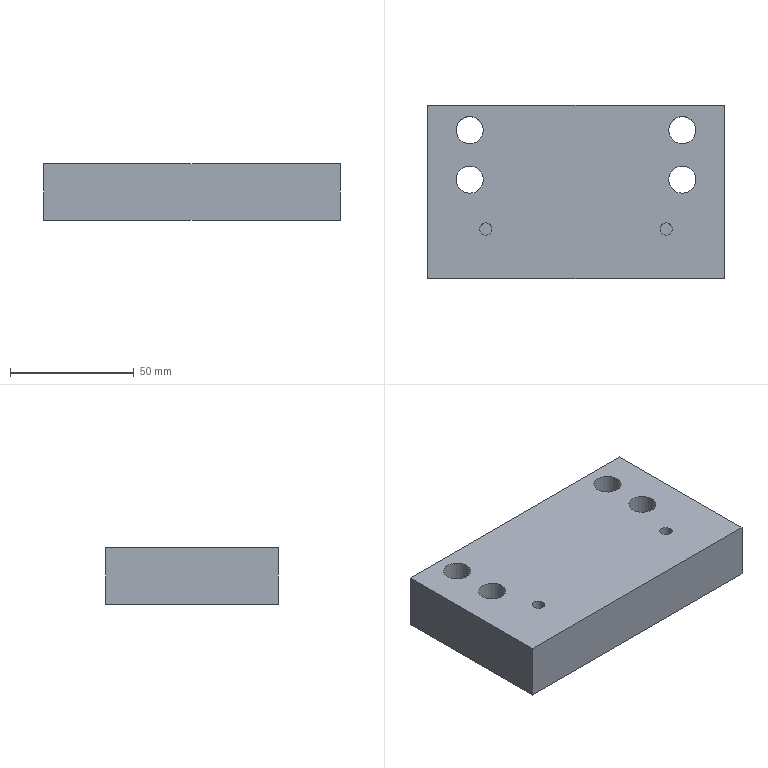Part | NX | features solid 2 | 1 solid | 14 faces | box 120 x 70 x 23 mm | volume 183672 mm3 | plane 8 | cylinder 6 | commonest cylinder face diameters 11 x4 5 x2
STEP:
#1=CARTESIAN_POINT('',(60.,440.,-40.));
#2=VERTEX_POINT('',#1);
#3=CARTESIAN_POINT('',(60.,510.,-40.));
#4=VERTEX_POINT('',#3);
#5=CARTESIAN_POINT('',(60.,425.,-40.));
#6=DIRECTION('',(0.,1.,0.));
#7=VECTOR('',#6,1000.);
#8=LINE('',#5,#7);
#9=EDGE_CURVE('',#2,#4,#8,.T.);
#10=ORIENTED_EDGE('',*,*,#9,.F.);
#11=CARTESIAN_POINT('',(60.,440.,-63.));
#12=VERTEX_POINT('',#11);
#13=CARTESIAN_POINT('',(60.,440.,-63.));
#14=DIRECTION('',(0.,0.,1.));
#15=VECTOR('',#14,1000.);
#16=LINE('',#13,#15);
#17=EDGE_CURVE('',#12,#2,#16,.T.);
#18=ORIENTED_EDGE('',*,*,#17,.F.);
#19=CARTESIAN_POINT('',(60.,510.,-63.));
#20=VERTEX_POINT('',#19);
#21=CARTESIAN_POINT('',(60.,425.,-63.));
#22=DIRECTION('',(0.,1.,0.));
#23=VECTOR('',#22,1000.);
#24=LINE('',#21,#23);
#25=EDGE_CURVE('',#12,#20,#24,.T.);
#26=ORIENTED_EDGE('',*,*,#25,.T.);
#27=CARTESIAN_POINT('',(60.,510.,-40.));
#28=DIRECTION('',(0.,0.,-1.));
#29=VECTOR('',#28,1000.);
#30=LINE('',#27,#29);
#31=EDGE_CURVE('',#4,#20,#30,.T.);
#32=ORIENTED_EDGE('',*,*,#31,.F.);
#33=EDGE_LOOP('',(#10,#18,#26,#32));
#34=FACE_BOUND('',#33,.T.);
#35=CARTESIAN_POINT('',(60.,-0.0135,0.));
#36=DIRECTION('',(1.,0.,0.));
#37=DIRECTION('',(0.,0.,-1.));
#38=AXIS2_PLACEMENT_3D('',#35,#36,#37);
#39=PLANE('',#38);
#40=ADVANCED_FACE('',(#34),#39,.T.);
#41=CARTESIAN_POINT('',(43.,505.5,-40.));
#42=VERTEX_POINT('',#41);
#43=CARTESIAN_POINT('',(43.,500.,-40.));
#44=DIRECTION('',(0.,0.,-1.));
#45=DIRECTION('',(0.,1.,0.));
#46=AXIS2_PLACEMENT_3D('',#43,#44,#45);
#47=CIRCLE('',#46,5.5);
#48=EDGE_CURVE('',#42,#42,#47,.T.);
#49=ORIENTED_EDGE('',*,*,#48,.F.);
#50=EDGE_LOOP('',(#49));
#51=FACE_BOUND('',#50,.T.);
#52=CARTESIAN_POINT('',(43.,494.5,-63.));
#53=VERTEX_POINT('',#52);
#54=CARTESIAN_POINT('',(43.,500.,-63.));
#55=DIRECTION('',(0.,0.,1.));
#56=DIRECTION('',(0.,-1.,0.));
#57=AXIS2_PLACEMENT_3D('',#54,#55,#56);
#58=CIRCLE('',#57,5.5);
#59=EDGE_CURVE('',#53,#53,#58,.T.);
#60=ORIENTED_EDGE('',*,*,#59,.F.);
#61=EDGE_LOOP('',(#60));
#62=FACE_BOUND('',#61,.T.);
#63=CARTESIAN_POINT('',(43.,500.,-40.));
#64=DIRECTION('',(0.,0.,-1.));
#65=DIRECTION('',(0.,1.,0.));
#66=AXIS2_PLACEMENT_3D('',#63,#64,#65);
#67=CYLINDRICAL_SURFACE('',#66,5.5);
#68=ADVANCED_FACE('',(#51,#62),#67,.F.);
#69=CARTESIAN_POINT('',(-43.,505.5,-40.));
#70=VERTEX_POINT('',#69);
#71=CARTESIAN_POINT('',(-43.,500.,-40.));
#72=DIRECTION('',(0.,0.,-1.));
#73=DIRECTION('',(0.,1.,0.));
#74=AXIS2_PLACEMENT_3D('',#71,#72,#73);
#75=CIRCLE('',#74,5.5);
#76=EDGE_CURVE('',#70,#70,#75,.T.);
#77=ORIENTED_EDGE('',*,*,#76,.F.);
#78=EDGE_LOOP('',(#77));
#79=FACE_BOUND('',#78,.T.);
#80=CARTESIAN_POINT('',(-43.,494.5,-63.));
#81=VERTEX_POINT('',#80);
#82=CARTESIAN_POINT('',(-43.,500.,-63.));
#83=DIRECTION('',(0.,0.,1.));
#84=DIRECTION('',(0.,-1.,0.));
#85=AXIS2_PLACEMENT_3D('',#82,#83,#84);
#86=CIRCLE('',#85,5.5);
#87=EDGE_CURVE('',#81,#81,#86,.T.);
#88=ORIENTED_EDGE('',*,*,#87,.F.);
#89=EDGE_LOOP('',(#88));
#90=FACE_BOUND('',#89,.T.);
#91=CARTESIAN_POINT('',(-43.,500.,-40.));
#92=DIRECTION('',(0.,0.,-1.));
#93=DIRECTION('',(0.,1.,0.));
#94=AXIS2_PLACEMENT_3D('',#91,#92,#93);
#95=CYLINDRICAL_SURFACE('',#94,5.5);
#96=ADVANCED_FACE('',(#79,#90),#95,.F.);
#97=CARTESIAN_POINT('',(43.,485.5,-40.));
#98=VERTEX_POINT('',#97);
#99=CARTESIAN_POINT('',(43.,480.,-40.));
#100=DIRECTION('',(0.,0.,-1.));
#101=DIRECTION('',(0.,1.,0.));
#102=AXIS2_PLACEMENT_3D('',#99,#100,#101);
#103=CIRCLE('',#102,5.5);
#104=EDGE_CURVE('',#98,#98,#103,.T.);
#105=ORIENTED_EDGE('',*,*,#104,.F.);
#106=EDGE_LOOP('',(#105));
#107=FACE_BOUND('',#106,.T.);
#108=CARTESIAN_POINT('',(43.,474.5,-63.));
#109=VERTEX_POINT('',#108);
#110=CARTESIAN_POINT('',(43.,480.,-63.));
#111=DIRECTION('',(0.,0.,1.));
#112=DIRECTION('',(0.,-1.,0.));
#113=AXIS2_PLACEMENT_3D('',#110,#111,#112);
#114=CIRCLE('',#113,5.5);
#115=EDGE_CURVE('',#109,#109,#114,.T.);
#116=ORIENTED_EDGE('',*,*,#115,.F.);
#117=EDGE_LOOP('',(#116));
#118=FACE_BOUND('',#117,.T.);
#119=CARTESIAN_POINT('',(43.,480.,-40.));
#120=DIRECTION('',(0.,0.,-1.));
#121=DIRECTION('',(0.,1.,0.));
#122=AXIS2_PLACEMENT_3D('',#119,#120,#121);
#123=CYLINDRICAL_SURFACE('',#122,5.5);
#124=ADVANCED_FACE('',(#107,#118),#123,.F.);
#125=CARTESIAN_POINT('',(-43.,485.5,-40.));
#126=VERTEX_POINT('',#125);
#127=CARTESIAN_POINT('',(-43.,480.,-40.));
#128=DIRECTION('',(0.,0.,-1.));
#129=DIRECTION('',(0.,1.,0.));
#130=AXIS2_PLACEMENT_3D('',#127,#128,#129);
#131=CIRCLE('',#130,5.5);
#132=EDGE_CURVE('',#126,#126,#131,.T.);
#133=ORIENTED_EDGE('',*,*,#132,.F.);
#134=EDGE_LOOP('',(#133));
#135=FACE_BOUND('',#134,.T.);
#136=CARTESIAN_POINT('',(-43.,474.5,-63.));
#137=VERTEX_POINT('',#136);
#138=CARTESIAN_POINT('',(-43.,480.,-63.));
#139=DIRECTION('',(0.,0.,1.));
#140=DIRECTION('',(0.,-1.,0.));
#141=AXIS2_PLACEMENT_3D('',#138,#139,#140);
#142=CIRCLE('',#141,5.5);
#143=EDGE_CURVE('',#137,#137,#142,.T.);
#144=ORIENTED_EDGE('',*,*,#143,.F.);
#145=EDGE_LOOP('',(#144));
#146=FACE_BOUND('',#145,.T.);
#147=CARTESIAN_POINT('',(-43.,480.,-40.));
#148=DIRECTION('',(0.,0.,-1.));
#149=DIRECTION('',(0.,1.,0.));
#150=AXIS2_PLACEMENT_3D('',#147,#148,#149);
#151=CYLINDRICAL_SURFACE('',#150,5.5);
#152=ADVANCED_FACE('',(#135,#146),#151,.F.);
#153=CARTESIAN_POINT('',(34.,460.,-40.));
#154=VERTEX_POINT('',#153);
#155=CARTESIAN_POINT('',(36.5,460.,-40.));
#156=DIRECTION('',(0.,0.,-1.));
#157=DIRECTION('',(-1.,0.,0.));
#158=AXIS2_PLACEMENT_3D('',#155,#156,#157);
#159=CIRCLE('',#158,2.5);
#160=EDGE_CURVE('',#154,#154,#159,.T.);
#161=ORIENTED_EDGE('',*,*,#160,.T.);
#162=EDGE_LOOP('',(#161));
#163=FACE_BOUND('',#162,.T.);
#164=CARTESIAN_POINT('',(-39.,460.,-40.));
#165=VERTEX_POINT('',#164);
#166=CARTESIAN_POINT('',(-36.5,460.,-40.));
#167=DIRECTION('',(0.,0.,-1.));
#168=DIRECTION('',(-1.,0.,0.));
#169=AXIS2_PLACEMENT_3D('',#166,#167,#168);
#170=CIRCLE('',#169,2.5);
#171=EDGE_CURVE('',#165,#165,#170,.T.);
#172=ORIENTED_EDGE('',*,*,#171,.T.);
#173=EDGE_LOOP('',(#172));
#174=FACE_BOUND('',#173,.T.);
#175=CARTESIAN_POINT('',(-60.,440.,-40.));
#176=VERTEX_POINT('',#175);
#177=CARTESIAN_POINT('',(-60.,510.,-40.));
#178=VERTEX_POINT('',#177);
#179=CARTESIAN_POINT('',(-60.,425.,-40.));
#180=DIRECTION('',(0.,1.,0.));
#181=VECTOR('',#180,1000.);
#182=LINE('',#179,#181);
#183=EDGE_CURVE('',#176,#178,#182,.T.);
#184=ORIENTED_EDGE('',*,*,#183,.F.);
#185=CARTESIAN_POINT('',(33.,440.,-40.));
#186=DIRECTION('',(-1.,0.,0.));
#187=VECTOR('',#186,1000.);
#188=LINE('',#185,#187);
#189=EDGE_CURVE('',#2,#176,#188,.T.);
#190=ORIENTED_EDGE('',*,*,#189,.F.);
#191=ORIENTED_EDGE('',*,*,#9,.T.);
#192=CARTESIAN_POINT('',(-90.,510.,-40.));
#193=DIRECTION('',(1.,0.,0.));
#194=VECTOR('',#193,1000.);
#195=LINE('',#192,#194);
#196=EDGE_CURVE('',#178,#4,#195,.T.);
#197=ORIENTED_EDGE('',*,*,#196,.F.);
#198=EDGE_LOOP('',(#184,#190,#191,#197));
#199=FACE_BOUND('',#198,.T.);
#200=ORIENTED_EDGE('',*,*,#132,.T.);
#201=EDGE_LOOP('',(#200));
#202=FACE_BOUND('',#201,.T.);
#203=ORIENTED_EDGE('',*,*,#104,.T.);
#204=EDGE_LOOP('',(#203));
#205=FACE_BOUND('',#204,.T.);
#206=ORIENTED_EDGE('',*,*,#76,.T.);
#207=EDGE_LOOP('',(#206));
#208=FACE_BOUND('',#207,.T.);
#209=ORIENTED_EDGE('',*,*,#48,.T.);
#210=EDGE_LOOP('',(#209));
#211=FACE_BOUND('',#210,.T.);
#212=CARTESIAN_POINT('',(-90.,425.,-40.));
#213=DIRECTION('',(0.,0.,1.));
#214=DIRECTION('',(0.,-1.,0.));
#215=AXIS2_PLACEMENT_3D('',#212,#213,#214);
#216=PLANE('',#215);
#217=ADVANCED_FACE('',(#163,#174,#199,#202,#205,#208,#211),#216,.T.);
#218=ORIENTED_EDGE('',*,*,#143,.T.);
#219=EDGE_LOOP('',(#218));
#220=FACE_BOUND('',#219,.T.);
#221=ORIENTED_EDGE('',*,*,#115,.T.);
#222=EDGE_LOOP('',(#221));
#223=FACE_BOUND('',#222,.T.);
#224=ORIENTED_EDGE('',*,*,#87,.T.);
#225=EDGE_LOOP('',(#224));
#226=FACE_BOUND('',#225,.T.);
#227=ORIENTED_EDGE('',*,*,#59,.T.);
#228=EDGE_LOOP('',(#227));
#229=FACE_BOUND('',#228,.T.);
#230=CARTESIAN_POINT('',(-60.,440.,-63.));
#231=VERTEX_POINT('',#230);
#232=CARTESIAN_POINT('',(33.,440.,-63.));
#233=DIRECTION('',(-1.,0.,0.));
#234=VECTOR('',#233,1000.);
#235=LINE('',#232,#234);
#236=EDGE_CURVE('',#12,#231,#235,.T.);
#237=ORIENTED_EDGE('',*,*,#236,.T.);
#238=CARTESIAN_POINT('',(-60.,510.,-63.));
#239=VERTEX_POINT('',#238);
#240=CARTESIAN_POINT('',(-60.,425.,-63.));
#241=DIRECTION('',(0.,1.,0.));
#242=VECTOR('',#241,1000.);
#243=LINE('',#240,#242);
#244=EDGE_CURVE('',#231,#239,#243,.T.);
#245=ORIENTED_EDGE('',*,*,#244,.T.);
#246=CARTESIAN_POINT('',(-90.,510.,-63.));
#247=DIRECTION('',(1.,0.,0.));
#248=VECTOR('',#247,1000.);
#249=LINE('',#246,#248);
#250=EDGE_CURVE('',#239,#20,#249,.T.);
#251=ORIENTED_EDGE('',*,*,#250,.T.);
#252=ORIENTED_EDGE('',*,*,#25,.F.);
#253=EDGE_LOOP('',(#237,#245,#251,#252));
#254=FACE_BOUND('',#253,.T.);
#255=CARTESIAN_POINT('',(-90.,425.,-63.));
#256=DIRECTION('',(0.,0.,1.));
#257=DIRECTION('',(0.,-1.,0.));
#258=AXIS2_PLACEMENT_3D('',#255,#256,#257);
#259=PLANE('',#258);
#260=ADVANCED_FACE('',(#220,#223,#226,#229,#254),#259,.F.);
#261=CARTESIAN_POINT('',(-60.,440.,-63.));
#262=DIRECTION('',(0.,0.,1.));
#263=VECTOR('',#262,1000.);
#264=LINE('',#261,#263);
#265=EDGE_CURVE('',#231,#176,#264,.T.);
#266=ORIENTED_EDGE('',*,*,#265,.F.);
#267=ORIENTED_EDGE('',*,*,#236,.F.);
#268=ORIENTED_EDGE('',*,*,#17,.T.);
#269=ORIENTED_EDGE('',*,*,#189,.T.);
#270=EDGE_LOOP('',(#266,#267,#268,#269));
#271=FACE_BOUND('',#270,.T.);
#272=CARTESIAN_POINT('',(33.,440.,-63.));
#273=DIRECTION('',(0.,-1.,0.));
#274=DIRECTION('',(0.,0.,-1.));
#275=AXIS2_PLACEMENT_3D('',#272,#273,#274);
#276=PLANE('',#275);
#277=ADVANCED_FACE('',(#271),#276,.T.);
#278=CARTESIAN_POINT('',(-60.,510.,-40.));
#279=DIRECTION('',(0.,0.,-1.));
#280=VECTOR('',#279,1000.);
#281=LINE('',#278,#280);
#282=EDGE_CURVE('',#178,#239,#281,.T.);
#283=ORIENTED_EDGE('',*,*,#282,.F.);
#284=ORIENTED_EDGE('',*,*,#196,.T.);
#285=ORIENTED_EDGE('',*,*,#31,.T.);
#286=ORIENTED_EDGE('',*,*,#250,.F.);
#287=EDGE_LOOP('',(#283,#284,#285,#286));
#288=FACE_BOUND('',#287,.T.);
#289=CARTESIAN_POINT('',(-90.,510.,-40.));
#290=DIRECTION('',(0.,1.,0.));
#291=DIRECTION('',(-1.,0.,0.));
#292=AXIS2_PLACEMENT_3D('',#289,#290,#291);
#293=PLANE('',#292);
#294=ADVANCED_FACE('',(#288),#293,.T.);
#295=ORIENTED_EDGE('',*,*,#183,.T.);
#296=ORIENTED_EDGE('',*,*,#282,.T.);
#297=ORIENTED_EDGE('',*,*,#244,.F.);
#298=ORIENTED_EDGE('',*,*,#265,.T.);
#299=EDGE_LOOP('',(#295,#296,#297,#298));
#300=FACE_BOUND('',#299,.T.);
#301=CARTESIAN_POINT('',(-60.,-0.0135,0.));
#302=DIRECTION('',(1.,0.,0.));
#303=DIRECTION('',(0.,0.,-1.));
#304=AXIS2_PLACEMENT_3D('',#301,#302,#303);
#305=PLANE('',#304);
#306=ADVANCED_FACE('',(#300),#305,.F.);
#307=CARTESIAN_POINT('',(-39.,460.,-60.));
#308=VERTEX_POINT('',#307);
#309=CARTESIAN_POINT('',(-36.5,460.,-60.));
#310=DIRECTION('',(0.,0.,-1.));
#311=DIRECTION('',(-1.,0.,0.));
#312=AXIS2_PLACEMENT_3D('',#309,#310,#311);
#313=CIRCLE('',#312,2.5);
#314=EDGE_CURVE('',#308,#308,#313,.T.);
#315=ORIENTED_EDGE('',*,*,#314,.F.);
#316=EDGE_LOOP('',(#315));
#317=FACE_BOUND('',#316,.T.);
#318=CARTESIAN_POINT('',(-36.5,460.,-60.));
#319=DIRECTION('',(0.,0.,-1.));
#320=DIRECTION('',(-1.,0.,0.));
#321=AXIS2_PLACEMENT_3D('',#318,#319,#320);
#322=PLANE('',#321);
#323=ADVANCED_FACE('',(#317),#322,.F.);
#324=ORIENTED_EDGE('',*,*,#314,.T.);
#325=EDGE_LOOP('',(#324));
#326=FACE_BOUND('',#325,.T.);
#327=ORIENTED_EDGE('',*,*,#171,.F.);
#328=EDGE_LOOP('',(#327));
#329=FACE_BOUND('',#328,.T.);
#330=CARTESIAN_POINT('',(-36.5,460.,-40.));
#331=DIRECTION('',(0.,0.,-1.));
#332=DIRECTION('',(-1.,0.,0.));
#333=AXIS2_PLACEMENT_3D('',#330,#331,#332);
#334=CYLINDRICAL_SURFACE('',#333,2.5);
#335=ADVANCED_FACE('',(#326,#329),#334,.F.);
#336=CARTESIAN_POINT('',(34.,460.,-60.));
#337=VERTEX_POINT('',#336);
#338=CARTESIAN_POINT('',(36.5,460.,-60.));
#339=DIRECTION('',(0.,0.,-1.));
#340=DIRECTION('',(-1.,0.,0.));
#341=AXIS2_PLACEMENT_3D('',#338,#339,#340);
#342=CIRCLE('',#341,2.5);
#343=EDGE_CURVE('',#337,#337,#342,.T.);
#344=ORIENTED_EDGE('',*,*,#343,.F.);
#345=EDGE_LOOP('',(#344));
#346=FACE_BOUND('',#345,.T.);
#347=CARTESIAN_POINT('',(36.5,460.,-60.));
#348=DIRECTION('',(0.,0.,-1.));
#349=DIRECTION('',(-1.,0.,0.));
#350=AXIS2_PLACEMENT_3D('',#347,#348,#349);
#351=PLANE('',#350);
#352=ADVANCED_FACE('',(#346),#351,.F.);
#353=ORIENTED_EDGE('',*,*,#343,.T.);
#354=EDGE_LOOP('',(#353));
#355=FACE_BOUND('',#354,.T.);
#356=ORIENTED_EDGE('',*,*,#160,.F.);
#357=EDGE_LOOP('',(#356));
#358=FACE_BOUND('',#357,.T.);
#359=CARTESIAN_POINT('',(36.5,460.,-40.));
#360=DIRECTION('',(0.,0.,-1.));
#361=DIRECTION('',(-1.,0.,0.));
#362=AXIS2_PLACEMENT_3D('',#359,#360,#361);
#363=CYLINDRICAL_SURFACE('',#362,2.5);
#364=ADVANCED_FACE('',(#355,#358),#363,.F.);
#365=CLOSED_SHELL('',(#40,#68,#96,#124,#152,#217,#260,#277,#294,#306,#323,#335,#352,#364));
#366=MANIFOLD_SOLID_BREP('',#365);
#367=(LENGTH_UNIT()NAMED_UNIT(*)SI_UNIT(.MILLI.,.METRE.));
#368=UNCERTAINTY_MEASURE_WITH_UNIT(LENGTH_MEASURE(0.00001),#367,'','');
#369=(NAMED_UNIT(*)PLANE_ANGLE_UNIT()SI_UNIT($,.RADIAN.));
#370=(NAMED_UNIT(*)SI_UNIT($,.STERADIAN.)SOLID_ANGLE_UNIT());
#371=(GEOMETRIC_REPRESENTATION_CONTEXT(3)GLOBAL_UNCERTAINTY_ASSIGNED_CONTEXT((#368))GLOBAL_UNIT_ASSIGNED_CONTEXT((#367,#369,#370))REPRESENTATION_CONTEXT('',''));
#372=ADVANCED_BREP_SHAPE_REPRESENTATION('',(#366),#371);